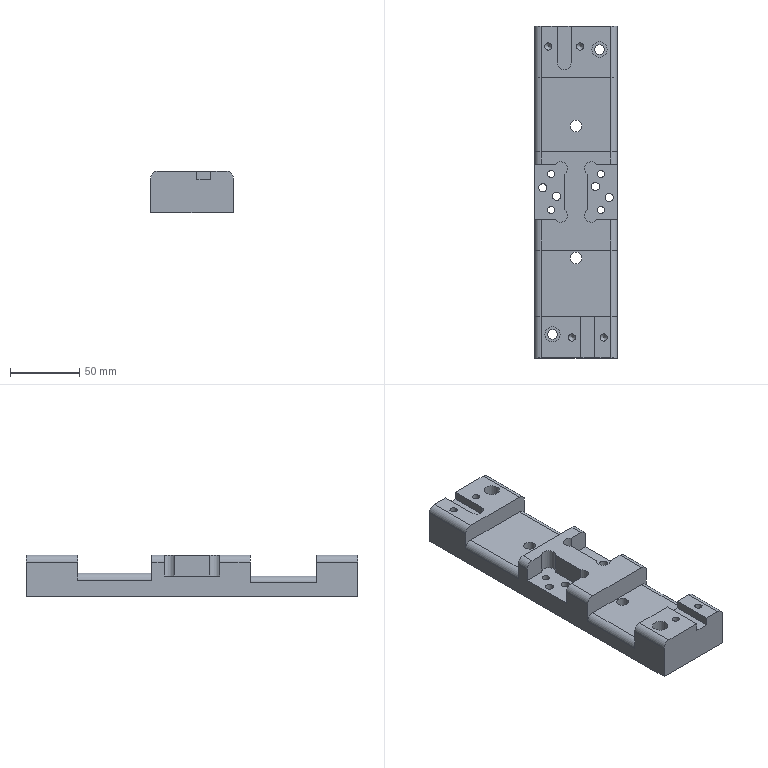Part | NX | features solid 2 | 1 solid | 78 faces | box 60 x 240 x 30 mm | volume 299038 mm3 | cylinder 39 | plane 35 | cone 4 | commonest cylinder face diameters 10 x17 5.2 x8 6.001 x4 6.799 x2 7 x2 8.5 x2